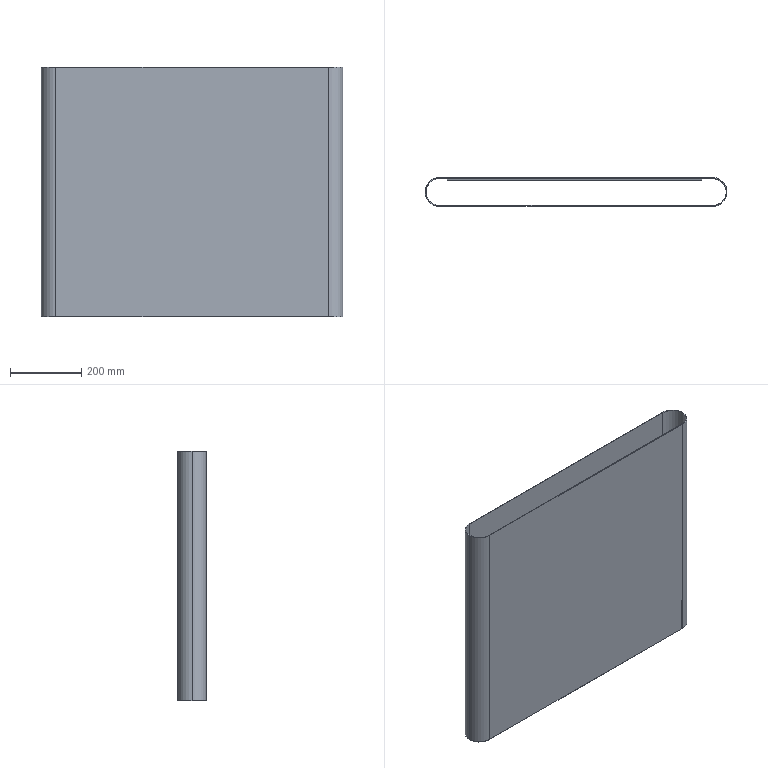Part | SolidWorks | features ExtruThin 1, ICE 1 | 1 solid | 17 faces | box 845 x 80 x 700 mm | volume 2508235 mm3 | plane 11 | cylinder 6 | commonest cylinder face diameters 76 x3 80 x3
STEP:
#1=CARTESIAN_POINT('',(-382.5,38.,350.));
#2=VERTEX_POINT('',#1);
#3=CARTESIAN_POINT('',(-420.5,0.,350.));
#4=VERTEX_POINT('',#3);
#5=CARTESIAN_POINT('',(-382.5,0.,350.));
#6=DIRECTION('',(0.,0.,1.));
#7=DIRECTION('',(1.,0.,0.));
#8=AXIS2_PLACEMENT_3D('',#5,#6,#7);
#9=CIRCLE('',#8,38.);
#10=EDGE_CURVE('',#2,#4,#9,.T.);
#11=ORIENTED_EDGE('',*,*,#10,.T.);
#12=CARTESIAN_POINT('',(-420.5,0.,-350.));
#13=VERTEX_POINT('',#12);
#14=CARTESIAN_POINT('',(-420.5,0.,350.));
#15=DIRECTION('',(0.,0.,-1.));
#16=VECTOR('',#15,1000.);
#17=LINE('',#14,#16);
#18=EDGE_CURVE('',#4,#13,#17,.T.);
#19=ORIENTED_EDGE('',*,*,#18,.T.);
#20=CARTESIAN_POINT('',(-382.5,38.,-350.));
#21=VERTEX_POINT('',#20);
#22=CARTESIAN_POINT('',(-382.5,0.,-350.));
#23=DIRECTION('',(0.,0.,1.));
#24=DIRECTION('',(1.,0.,0.));
#25=AXIS2_PLACEMENT_3D('',#22,#23,#24);
#26=CIRCLE('',#25,38.);
#27=EDGE_CURVE('',#21,#13,#26,.T.);
#28=ORIENTED_EDGE('',*,*,#27,.F.);
#29=CARTESIAN_POINT('',(-382.5,38.,350.));
#30=DIRECTION('',(0.,0.,-1.));
#31=VECTOR('',#30,1000.);
#32=LINE('',#29,#31);
#33=EDGE_CURVE('',#2,#21,#32,.T.);
#34=ORIENTED_EDGE('',*,*,#33,.F.);
#35=EDGE_LOOP('',(#11,#19,#28,#34));
#36=FACE_OUTER_BOUND('',#35,.T.);
#37=CARTESIAN_POINT('',(-382.5,0.,350.));
#38=DIRECTION('',(0.,0.,-1.));
#39=DIRECTION('',(-1.,0.,0.));
#40=AXIS2_PLACEMENT_3D('',#37,#38,#39);
#41=CYLINDRICAL_SURFACE('',#40,38.);
#42=ADVANCED_FACE('',(#36),#41,.F.);
#43=CARTESIAN_POINT('',(-422.5,0.,350.));
#44=VERTEX_POINT('',#43);
#45=CARTESIAN_POINT('',(-381.234,-39.98,350.));
#46=VERTEX_POINT('',#45);
#47=CARTESIAN_POINT('',(-382.5,0.,350.));
#48=DIRECTION('',(0.,0.,1.));
#49=DIRECTION('',(1.,0.,0.));
#50=AXIS2_PLACEMENT_3D('',#47,#48,#49);
#51=CIRCLE('',#50,40.);
#52=EDGE_CURVE('',#44,#46,#51,.T.);
#53=ORIENTED_EDGE('',*,*,#52,.F.);
#54=CARTESIAN_POINT('',(-422.5,0.,-350.));
#55=VERTEX_POINT('',#54);
#56=CARTESIAN_POINT('',(-422.5,0.,350.));
#57=DIRECTION('',(0.,0.,-1.));
#58=VECTOR('',#57,1000.);
#59=LINE('',#56,#58);
#60=EDGE_CURVE('',#44,#55,#59,.T.);
#61=ORIENTED_EDGE('',*,*,#60,.T.);
#62=CARTESIAN_POINT('',(-381.234,-39.98,-350.));
#63=VERTEX_POINT('',#62);
#64=CARTESIAN_POINT('',(-382.5,0.,-350.));
#65=DIRECTION('',(0.,0.,1.));
#66=DIRECTION('',(1.,0.,0.));
#67=AXIS2_PLACEMENT_3D('',#64,#65,#66);
#68=CIRCLE('',#67,40.);
#69=EDGE_CURVE('',#55,#63,#68,.T.);
#70=ORIENTED_EDGE('',*,*,#69,.T.);
#71=CARTESIAN_POINT('',(-381.234,-39.98,350.));
#72=DIRECTION('',(0.,0.,-1.));
#73=VECTOR('',#72,1000.);
#74=LINE('',#71,#73);
#75=EDGE_CURVE('',#46,#63,#74,.T.);
#76=ORIENTED_EDGE('',*,*,#75,.F.);
#77=EDGE_LOOP('',(#53,#61,#70,#76));
#78=FACE_OUTER_BOUND('',#77,.T.);
#79=CARTESIAN_POINT('',(-382.5,0.,350.));
#80=DIRECTION('',(0.,0.,-1.));
#81=DIRECTION('',(-1.,0.,0.));
#82=AXIS2_PLACEMENT_3D('',#79,#80,#81);
#83=CYLINDRICAL_SURFACE('',#82,40.);
#84=ADVANCED_FACE('',(#78),#83,.T.);
#85=CARTESIAN_POINT('',(382.5,38.,-350.));
#86=VERTEX_POINT('',#85);
#87=CARTESIAN_POINT('',(-382.5,38.,-350.));
#88=DIRECTION('',(-1.,0.,0.));
#89=VECTOR('',#88,1000.);
#90=LINE('',#87,#89);
#91=EDGE_CURVE('',#86,#21,#90,.T.);
#92=ORIENTED_EDGE('',*,*,#91,.F.);
#93=CARTESIAN_POINT('',(382.5,38.,350.));
#94=VERTEX_POINT('',#93);
#95=CARTESIAN_POINT('',(382.5,38.,350.));
#96=DIRECTION('',(0.,0.,-1.));
#97=VECTOR('',#96,1000.);
#98=LINE('',#95,#97);
#99=EDGE_CURVE('',#94,#86,#98,.T.);
#100=ORIENTED_EDGE('',*,*,#99,.F.);
#101=CARTESIAN_POINT('',(-382.5,38.,350.));
#102=DIRECTION('',(-1.,0.,0.));
#103=VECTOR('',#102,1000.);
#104=LINE('',#101,#103);
#105=EDGE_CURVE('',#94,#2,#104,.T.);
#106=ORIENTED_EDGE('',*,*,#105,.T.);
#107=ORIENTED_EDGE('',*,*,#33,.T.);
#108=EDGE_LOOP('',(#92,#100,#106,#107));
#109=FACE_OUTER_BOUND('',#108,.T.);
#110=CARTESIAN_POINT('',(-361.,38.,-4.));
#111=VERTEX_POINT('',#110);
#112=CARTESIAN_POINT('',(352.,38.,-4.));
#113=VERTEX_POINT('',#112);
#114=CARTESIAN_POINT('',(-361.,38.,-4.));
#115=DIRECTION('',(1.,0.,0.));
#116=VECTOR('',#115,1000.);
#117=LINE('',#114,#116);
#118=EDGE_CURVE('',#111,#113,#117,.T.);
#119=ORIENTED_EDGE('',*,*,#118,.F.);
#120=CARTESIAN_POINT('',(-361.,38.,4.));
#121=VERTEX_POINT('',#120);
#122=CARTESIAN_POINT('',(-361.,38.,-4.));
#123=DIRECTION('',(0.,0.,1.));
#124=VECTOR('',#123,1000.);
#125=LINE('',#122,#124);
#126=EDGE_CURVE('',#111,#121,#125,.T.);
#127=ORIENTED_EDGE('',*,*,#126,.T.);
#128=CARTESIAN_POINT('',(352.,38.,4.));
#129=VERTEX_POINT('',#128);
#130=CARTESIAN_POINT('',(-361.,38.,4.));
#131=DIRECTION('',(1.,0.,0.));
#132=VECTOR('',#131,1000.);
#133=LINE('',#130,#132);
#134=EDGE_CURVE('',#121,#129,#133,.T.);
#135=ORIENTED_EDGE('',*,*,#134,.T.);
#136=CARTESIAN_POINT('',(352.,38.,-4.));
#137=DIRECTION('',(0.,0.,1.));
#138=VECTOR('',#137,1000.);
#139=LINE('',#136,#138);
#140=EDGE_CURVE('',#113,#129,#139,.T.);
#141=ORIENTED_EDGE('',*,*,#140,.F.);
#142=EDGE_LOOP('',(#119,#127,#135,#141));
#143=FACE_BOUND('',#142,.T.);
#144=CARTESIAN_POINT('',(-382.5,38.,350.));
#145=DIRECTION('',(0.,-1.,0.));
#146=DIRECTION('',(0.,0.,-1.));
#147=AXIS2_PLACEMENT_3D('',#144,#145,#146);
#148=PLANE('',#147);
#149=ADVANCED_FACE('',(#109,#143),#148,.T.);
#150=CARTESIAN_POINT('',(-382.5,40.,350.));
#151=VERTEX_POINT('',#150);
#152=CARTESIAN_POINT('',(-382.5,0.,350.));
#153=DIRECTION('',(0.,0.,1.));
#154=DIRECTION('',(1.,0.,0.));
#155=AXIS2_PLACEMENT_3D('',#152,#153,#154);
#156=CIRCLE('',#155,40.);
#157=EDGE_CURVE('',#151,#44,#156,.T.);
#158=ORIENTED_EDGE('',*,*,#157,.T.);
#159=ORIENTED_EDGE('',*,*,#52,.T.);
#160=CARTESIAN_POINT('',(381.234,-39.98,350.));
#161=VERTEX_POINT('',#160);
#162=CARTESIAN_POINT('',(381.266,-39.98,350.));
#163=DIRECTION('',(1.,0.,0.));
#164=VECTOR('',#163,1000.);
#165=LINE('',#162,#164);
#166=EDGE_CURVE('',#46,#161,#165,.T.);
#167=ORIENTED_EDGE('',*,*,#166,.T.);
#168=CARTESIAN_POINT('',(382.5,40.,350.));
#169=VERTEX_POINT('',#168);
#170=CARTESIAN_POINT('',(382.5,0.,350.));
#171=DIRECTION('',(0.,0.,1.));
#172=DIRECTION('',(1.,0.,0.));
#173=AXIS2_PLACEMENT_3D('',#170,#171,#172);
#174=CIRCLE('',#173,40.);
#175=EDGE_CURVE('',#161,#169,#174,.T.);
#176=ORIENTED_EDGE('',*,*,#175,.T.);
#177=CARTESIAN_POINT('',(-382.5,40.,350.));
#178=DIRECTION('',(-1.,0.,0.));
#179=VECTOR('',#178,1000.);
#180=LINE('',#177,#179);
#181=EDGE_CURVE('',#169,#151,#180,.T.);
#182=ORIENTED_EDGE('',*,*,#181,.T.);
#183=EDGE_LOOP('',(#158,#159,#167,#176,#182));
#184=FACE_OUTER_BOUND('',#183,.T.);
#185=CARTESIAN_POINT('',(-381.266,-37.98,350.));
#186=VERTEX_POINT('',#185);
#187=CARTESIAN_POINT('',(381.266,-37.98,350.));
#188=VERTEX_POINT('',#187);
#189=CARTESIAN_POINT('',(381.266,-37.98,350.));
#190=DIRECTION('',(1.,0.,0.));
#191=VECTOR('',#190,1000.);
#192=LINE('',#189,#191);
#193=EDGE_CURVE('',#186,#188,#192,.T.);
#194=ORIENTED_EDGE('',*,*,#193,.F.);
#195=CARTESIAN_POINT('',(-382.5,0.,350.));
#196=DIRECTION('',(0.,0.,1.));
#197=DIRECTION('',(1.,0.,0.));
#198=AXIS2_PLACEMENT_3D('',#195,#196,#197);
#199=CIRCLE('',#198,38.);
#200=EDGE_CURVE('',#4,#186,#199,.T.);
#201=ORIENTED_EDGE('',*,*,#200,.F.);
#202=ORIENTED_EDGE('',*,*,#10,.F.);
#203=ORIENTED_EDGE('',*,*,#105,.F.);
#204=CARTESIAN_POINT('',(382.5,0.,350.));
#205=DIRECTION('',(0.,0.,1.));
#206=DIRECTION('',(1.,0.,0.));
#207=AXIS2_PLACEMENT_3D('',#204,#205,#206);
#208=CIRCLE('',#207,38.);
#209=EDGE_CURVE('',#188,#94,#208,.T.);
#210=ORIENTED_EDGE('',*,*,#209,.F.);
#211=EDGE_LOOP('',(#194,#201,#202,#203,#210));
#212=FACE_BOUND('',#211,.T.);
#213=CARTESIAN_POINT('',(-382.5,0.,350.));
#214=DIRECTION('',(0.,0.,1.));
#215=DIRECTION('',(1.,0.,0.));
#216=AXIS2_PLACEMENT_3D('',#213,#214,#215);
#217=PLANE('',#216);
#218=ADVANCED_FACE('',(#184,#212),#217,.T.);
#219=CARTESIAN_POINT('',(-382.5,40.,-350.));
#220=VERTEX_POINT('',#219);
#221=CARTESIAN_POINT('',(-382.5,0.,-350.));
#222=DIRECTION('',(0.,0.,1.));
#223=DIRECTION('',(1.,0.,0.));
#224=AXIS2_PLACEMENT_3D('',#221,#222,#223);
#225=CIRCLE('',#224,40.);
#226=EDGE_CURVE('',#220,#55,#225,.T.);
#227=ORIENTED_EDGE('',*,*,#226,.F.);
#228=CARTESIAN_POINT('',(382.5,40.,-350.));
#229=VERTEX_POINT('',#228);
#230=CARTESIAN_POINT('',(-382.5,40.,-350.));
#231=DIRECTION('',(-1.,0.,0.));
#232=VECTOR('',#231,1000.);
#233=LINE('',#230,#232);
#234=EDGE_CURVE('',#229,#220,#233,.T.);
#235=ORIENTED_EDGE('',*,*,#234,.F.);
#236=CARTESIAN_POINT('',(381.234,-39.98,-350.));
#237=VERTEX_POINT('',#236);
#238=CARTESIAN_POINT('',(382.5,0.,-350.));
#239=DIRECTION('',(0.,0.,1.));
#240=DIRECTION('',(1.,0.,0.));
#241=AXIS2_PLACEMENT_3D('',#238,#239,#240);
#242=CIRCLE('',#241,40.);
#243=EDGE_CURVE('',#237,#229,#242,.T.);
#244=ORIENTED_EDGE('',*,*,#243,.F.);
#245=CARTESIAN_POINT('',(381.266,-39.98,-350.));
#246=DIRECTION('',(1.,0.,0.));
#247=VECTOR('',#246,1000.);
#248=LINE('',#245,#247);
#249=EDGE_CURVE('',#63,#237,#248,.T.);
#250=ORIENTED_EDGE('',*,*,#249,.F.);
#251=ORIENTED_EDGE('',*,*,#69,.F.);
#252=EDGE_LOOP('',(#227,#235,#244,#250,#251));
#253=FACE_OUTER_BOUND('',#252,.T.);
#254=ORIENTED_EDGE('',*,*,#27,.T.);
#255=CARTESIAN_POINT('',(-381.266,-37.98,-350.));
#256=VERTEX_POINT('',#255);
#257=CARTESIAN_POINT('',(-382.5,0.,-350.));
#258=DIRECTION('',(0.,0.,1.));
#259=DIRECTION('',(1.,0.,0.));
#260=AXIS2_PLACEMENT_3D('',#257,#258,#259);
#261=CIRCLE('',#260,38.);
#262=EDGE_CURVE('',#13,#256,#261,.T.);
#263=ORIENTED_EDGE('',*,*,#262,.T.);
#264=CARTESIAN_POINT('',(381.266,-37.98,-350.));
#265=VERTEX_POINT('',#264);
#266=CARTESIAN_POINT('',(381.266,-37.98,-350.));
#267=DIRECTION('',(1.,0.,0.));
#268=VECTOR('',#267,1000.);
#269=LINE('',#266,#268);
#270=EDGE_CURVE('',#256,#265,#269,.T.);
#271=ORIENTED_EDGE('',*,*,#270,.T.);
#272=CARTESIAN_POINT('',(382.5,0.,-350.));
#273=DIRECTION('',(0.,0.,1.));
#274=DIRECTION('',(1.,0.,0.));
#275=AXIS2_PLACEMENT_3D('',#272,#273,#274);
#276=CIRCLE('',#275,38.);
#277=EDGE_CURVE('',#265,#86,#276,.T.);
#278=ORIENTED_EDGE('',*,*,#277,.T.);
#279=ORIENTED_EDGE('',*,*,#91,.T.);
#280=EDGE_LOOP('',(#254,#263,#271,#278,#279));
#281=FACE_BOUND('',#280,.T.);
#282=CARTESIAN_POINT('',(-382.5,0.,-350.));
#283=DIRECTION('',(0.,0.,1.));
#284=DIRECTION('',(1.,0.,0.));
#285=AXIS2_PLACEMENT_3D('',#282,#283,#284);
#286=PLANE('',#285);
#287=ADVANCED_FACE('',(#253,#281),#286,.F.);
#288=ORIENTED_EDGE('',*,*,#60,.F.);
#289=ORIENTED_EDGE('',*,*,#157,.F.);
#290=CARTESIAN_POINT('',(-382.5,40.,350.));
#291=DIRECTION('',(0.,0.,-1.));
#292=VECTOR('',#291,1000.);
#293=LINE('',#290,#292);
#294=EDGE_CURVE('',#151,#220,#293,.T.);
#295=ORIENTED_EDGE('',*,*,#294,.T.);
#296=ORIENTED_EDGE('',*,*,#226,.T.);
#297=EDGE_LOOP('',(#288,#289,#295,#296));
#298=FACE_OUTER_BOUND('',#297,.T.);
#299=CARTESIAN_POINT('',(-382.5,0.,350.));
#300=DIRECTION('',(0.,0.,-1.));
#301=DIRECTION('',(-1.,0.,0.));
#302=AXIS2_PLACEMENT_3D('',#299,#300,#301);
#303=CYLINDRICAL_SURFACE('',#302,40.);
#304=ADVANCED_FACE('',(#298),#303,.T.);
#305=ORIENTED_EDGE('',*,*,#249,.T.);
#306=CARTESIAN_POINT('',(381.234,-39.98,350.));
#307=DIRECTION('',(0.,0.,-1.));
#308=VECTOR('',#307,1000.);
#309=LINE('',#306,#308);
#310=EDGE_CURVE('',#161,#237,#309,.T.);
#311=ORIENTED_EDGE('',*,*,#310,.F.);
#312=ORIENTED_EDGE('',*,*,#166,.F.);
#313=ORIENTED_EDGE('',*,*,#75,.T.);
#314=EDGE_LOOP('',(#305,#311,#312,#313));
#315=FACE_OUTER_BOUND('',#314,.T.);
#316=CARTESIAN_POINT('',(381.266,-39.98,350.));
#317=DIRECTION('',(0.,1.,0.));
#318=DIRECTION('',(-1.,0.,0.));
#319=AXIS2_PLACEMENT_3D('',#316,#317,#318);
#320=PLANE('',#319);
#321=ADVANCED_FACE('',(#315),#320,.F.);
#322=ORIENTED_EDGE('',*,*,#243,.T.);
#323=CARTESIAN_POINT('',(382.5,40.,350.));
#324=DIRECTION('',(0.,0.,-1.));
#325=VECTOR('',#324,1000.);
#326=LINE('',#323,#325);
#327=EDGE_CURVE('',#169,#229,#326,.T.);
#328=ORIENTED_EDGE('',*,*,#327,.F.);
#329=ORIENTED_EDGE('',*,*,#175,.F.);
#330=ORIENTED_EDGE('',*,*,#310,.T.);
#331=EDGE_LOOP('',(#322,#328,#329,#330));
#332=FACE_OUTER_BOUND('',#331,.T.);
#333=CARTESIAN_POINT('',(382.5,0.,350.));
#334=DIRECTION('',(0.,0.,-1.));
#335=DIRECTION('',(-1.,0.,0.));
#336=AXIS2_PLACEMENT_3D('',#333,#334,#335);
#337=CYLINDRICAL_SURFACE('',#336,40.);
#338=ADVANCED_FACE('',(#332),#337,.T.);
#339=ORIENTED_EDGE('',*,*,#234,.T.);
#340=ORIENTED_EDGE('',*,*,#294,.F.);
#341=ORIENTED_EDGE('',*,*,#181,.F.);
#342=ORIENTED_EDGE('',*,*,#327,.T.);
#343=EDGE_LOOP('',(#339,#340,#341,#342));
#344=FACE_OUTER_BOUND('',#343,.T.);
#345=CARTESIAN_POINT('',(-382.5,40.,350.));
#346=DIRECTION('',(0.,-1.,0.));
#347=DIRECTION('',(0.,0.,-1.));
#348=AXIS2_PLACEMENT_3D('',#345,#346,#347);
#349=PLANE('',#348);
#350=ADVANCED_FACE('',(#344),#349,.F.);
#351=ORIENTED_EDGE('',*,*,#18,.F.);
#352=ORIENTED_EDGE('',*,*,#200,.T.);
#353=CARTESIAN_POINT('',(-381.266,-37.98,350.));
#354=DIRECTION('',(0.,0.,-1.));
#355=VECTOR('',#354,1000.);
#356=LINE('',#353,#355);
#357=EDGE_CURVE('',#186,#256,#356,.T.);
#358=ORIENTED_EDGE('',*,*,#357,.T.);
#359=ORIENTED_EDGE('',*,*,#262,.F.);
#360=EDGE_LOOP('',(#351,#352,#358,#359));
#361=FACE_OUTER_BOUND('',#360,.T.);
#362=CARTESIAN_POINT('',(-382.5,0.,350.));
#363=DIRECTION('',(0.,0.,-1.));
#364=DIRECTION('',(-1.,0.,0.));
#365=AXIS2_PLACEMENT_3D('',#362,#363,#364);
#366=CYLINDRICAL_SURFACE('',#365,38.);
#367=ADVANCED_FACE('',(#361),#366,.F.);
#368=ORIENTED_EDGE('',*,*,#270,.F.);
#369=ORIENTED_EDGE('',*,*,#357,.F.);
#370=ORIENTED_EDGE('',*,*,#193,.T.);
#371=CARTESIAN_POINT('',(381.266,-37.98,350.));
#372=DIRECTION('',(0.,0.,-1.));
#373=VECTOR('',#372,1000.);
#374=LINE('',#371,#373);
#375=EDGE_CURVE('',#188,#265,#374,.T.);
#376=ORIENTED_EDGE('',*,*,#375,.T.);
#377=EDGE_LOOP('',(#368,#369,#370,#376));
#378=FACE_OUTER_BOUND('',#377,.T.);
#379=CARTESIAN_POINT('',(381.266,-37.98,350.));
#380=DIRECTION('',(0.,1.,0.));
#381=DIRECTION('',(-1.,0.,0.));
#382=AXIS2_PLACEMENT_3D('',#379,#380,#381);
#383=PLANE('',#382);
#384=ADVANCED_FACE('',(#378),#383,.T.);
#385=ORIENTED_EDGE('',*,*,#277,.F.);
#386=ORIENTED_EDGE('',*,*,#375,.F.);
#387=ORIENTED_EDGE('',*,*,#209,.T.);
#388=ORIENTED_EDGE('',*,*,#99,.T.);
#389=EDGE_LOOP('',(#385,#386,#387,#388));
#390=FACE_OUTER_BOUND('',#389,.T.);
#391=CARTESIAN_POINT('',(382.5,0.,350.));
#392=DIRECTION('',(0.,0.,-1.));
#393=DIRECTION('',(-1.,0.,0.));
#394=AXIS2_PLACEMENT_3D('',#391,#392,#393);
#395=CYLINDRICAL_SURFACE('',#394,38.);
#396=ADVANCED_FACE('',(#390),#395,.F.);
#397=CARTESIAN_POINT('',(-361.,33.,2.5));
#398=VERTEX_POINT('',#397);
#399=CARTESIAN_POINT('',(352.,33.,2.5));
#400=VERTEX_POINT('',#399);
#401=CARTESIAN_POINT('',(-361.,33.,2.5));
#402=DIRECTION('',(1.,0.,0.));
#403=VECTOR('',#402,1000.);
#404=LINE('',#401,#403);
#405=EDGE_CURVE('',#398,#400,#404,.T.);
#406=ORIENTED_EDGE('',*,*,#405,.T.);
#407=CARTESIAN_POINT('',(352.,38.,4.));
#408=DIRECTION('',(0.,-0.9578,-0.2873));
#409=VECTOR('',#408,1000.);
#410=LINE('',#407,#409);
#411=EDGE_CURVE('',#129,#400,#410,.T.);
#412=ORIENTED_EDGE('',*,*,#411,.F.);
#413=ORIENTED_EDGE('',*,*,#134,.F.);
#414=CARTESIAN_POINT('',(-361.,38.,4.));
#415=DIRECTION('',(0.,-0.9578,-0.2873));
#416=VECTOR('',#415,1000.);
#417=LINE('',#414,#416);
#418=EDGE_CURVE('',#121,#398,#417,.T.);
#419=ORIENTED_EDGE('',*,*,#418,.T.);
#420=EDGE_LOOP('',(#406,#412,#413,#419));
#421=FACE_OUTER_BOUND('',#420,.T.);
#422=CARTESIAN_POINT('',(-361.,38.,4.));
#423=DIRECTION('',(0.,-0.2873,0.9578));
#424=DIRECTION('',(0.,-0.9578,-0.2873));
#425=AXIS2_PLACEMENT_3D('',#422,#423,#424);
#426=PLANE('',#425);
#427=ADVANCED_FACE('',(#421),#426,.T.);
#428=ORIENTED_EDGE('',*,*,#118,.T.);
#429=CARTESIAN_POINT('',(352.,33.,-2.5));
#430=VERTEX_POINT('',#429);
#431=CARTESIAN_POINT('',(352.,38.,-4.));
#432=DIRECTION('',(0.,0.9578,-0.2873));
#433=VECTOR('',#432,1000.);
#434=LINE('',#431,#433);
#435=EDGE_CURVE('',#430,#113,#434,.T.);
#436=ORIENTED_EDGE('',*,*,#435,.F.);
#437=CARTESIAN_POINT('',(-361.,33.,-2.5));
#438=VERTEX_POINT('',#437);
#439=CARTESIAN_POINT('',(-361.,33.,-2.5));
#440=DIRECTION('',(1.,0.,0.));
#441=VECTOR('',#440,1000.);
#442=LINE('',#439,#441);
#443=EDGE_CURVE('',#438,#430,#442,.T.);
#444=ORIENTED_EDGE('',*,*,#443,.F.);
#445=CARTESIAN_POINT('',(-361.,38.,-4.));
#446=DIRECTION('',(0.,0.9578,-0.2873));
#447=VECTOR('',#446,1000.);
#448=LINE('',#445,#447);
#449=EDGE_CURVE('',#438,#111,#448,.T.);
#450=ORIENTED_EDGE('',*,*,#449,.T.);
#451=EDGE_LOOP('',(#428,#436,#444,#450));
#452=FACE_OUTER_BOUND('',#451,.T.);
#453=CARTESIAN_POINT('',(-361.,38.,-4.));
#454=DIRECTION('',(0.,-0.2873,-0.9578));
#455=DIRECTION('',(0.,0.9578,-0.2873));
#456=AXIS2_PLACEMENT_3D('',#453,#454,#455);
#457=PLANE('',#456);
#458=ADVANCED_FACE('',(#452),#457,.T.);
#459=ORIENTED_EDGE('',*,*,#443,.T.);
#460=CARTESIAN_POINT('',(352.,33.,2.5));
#461=DIRECTION('',(0.,0.,-1.));
#462=VECTOR('',#461,1000.);
#463=LINE('',#460,#462);
#464=EDGE_CURVE('',#400,#430,#463,.T.);
#465=ORIENTED_EDGE('',*,*,#464,.F.);
#466=ORIENTED_EDGE('',*,*,#405,.F.);
#467=CARTESIAN_POINT('',(-361.,33.,2.5));
#468=DIRECTION('',(0.,0.,-1.));
#469=VECTOR('',#468,1000.);
#470=LINE('',#467,#469);
#471=EDGE_CURVE('',#398,#438,#470,.T.);
#472=ORIENTED_EDGE('',*,*,#471,.T.);
#473=EDGE_LOOP('',(#459,#465,#466,#472));
#474=FACE_OUTER_BOUND('',#473,.T.);
#475=CARTESIAN_POINT('',(-361.,33.,2.5));
#476=DIRECTION('',(0.,-1.,0.));
#477=DIRECTION('',(0.,0.,-1.));
#478=AXIS2_PLACEMENT_3D('',#475,#476,#477);
#479=PLANE('',#478);
#480=ADVANCED_FACE('',(#474),#479,.T.);
#481=ORIENTED_EDGE('',*,*,#418,.F.);
#482=ORIENTED_EDGE('',*,*,#126,.F.);
#483=ORIENTED_EDGE('',*,*,#449,.F.);
#484=ORIENTED_EDGE('',*,*,#471,.F.);
#485=EDGE_LOOP('',(#481,#482,#483,#484));
#486=FACE_OUTER_BOUND('',#485,.T.);
#487=CARTESIAN_POINT('',(-361.,0.,0.));
#488=DIRECTION('',(1.,0.,0.));
#489=DIRECTION('',(0.,0.,-1.));
#490=AXIS2_PLACEMENT_3D('',#487,#488,#489);
#491=PLANE('',#490);
#492=ADVANCED_FACE('',(#486),#491,.F.);
#493=ORIENTED_EDGE('',*,*,#411,.T.);
#494=ORIENTED_EDGE('',*,*,#464,.T.);
#495=ORIENTED_EDGE('',*,*,#435,.T.);
#496=ORIENTED_EDGE('',*,*,#140,.T.);
#497=EDGE_LOOP('',(#493,#494,#495,#496));
#498=FACE_OUTER_BOUND('',#497,.T.);
#499=CARTESIAN_POINT('',(352.,0.,0.));
#500=DIRECTION('',(1.,0.,0.));
#501=DIRECTION('',(0.,0.,-1.));
#502=AXIS2_PLACEMENT_3D('',#499,#500,#501);
#503=PLANE('',#502);
#504=ADVANCED_FACE('',(#498),#503,.T.);
#505=CLOSED_SHELL('',(#42,#84,#149,#218,#287,#304,#321,#338,#350,#367,#384,#396,#427,#458,#480,#492,#504));
#506=MANIFOLD_SOLID_BREP('',#505);
#507=CARTESIAN_POINT('',(0.,0.,0.));
#508=DIRECTION('',(0.,0.,1.));
#509=DIRECTION('',(1.,0.,0.));
#510=AXIS2_PLACEMENT_3D('',#507,#508,#509);
#511=(LENGTH_UNIT()NAMED_UNIT(*)SI_UNIT(.MILLI.,.METRE.));
#512=UNCERTAINTY_MEASURE_WITH_UNIT(LENGTH_MEASURE(0.00001),#511,'','');
#513=(NAMED_UNIT(*)PLANE_ANGLE_UNIT()SI_UNIT($,.RADIAN.));
#514=(NAMED_UNIT(*)SI_UNIT($,.STERADIAN.)SOLID_ANGLE_UNIT());
#515=(GEOMETRIC_REPRESENTATION_CONTEXT(3)GLOBAL_UNCERTAINTY_ASSIGNED_CONTEXT((#512))GLOBAL_UNIT_ASSIGNED_CONTEXT((#511,#513,#514))REPRESENTATION_CONTEXT('',''));
#516=ADVANCED_BREP_SHAPE_REPRESENTATION('',(#506,#510),#515);